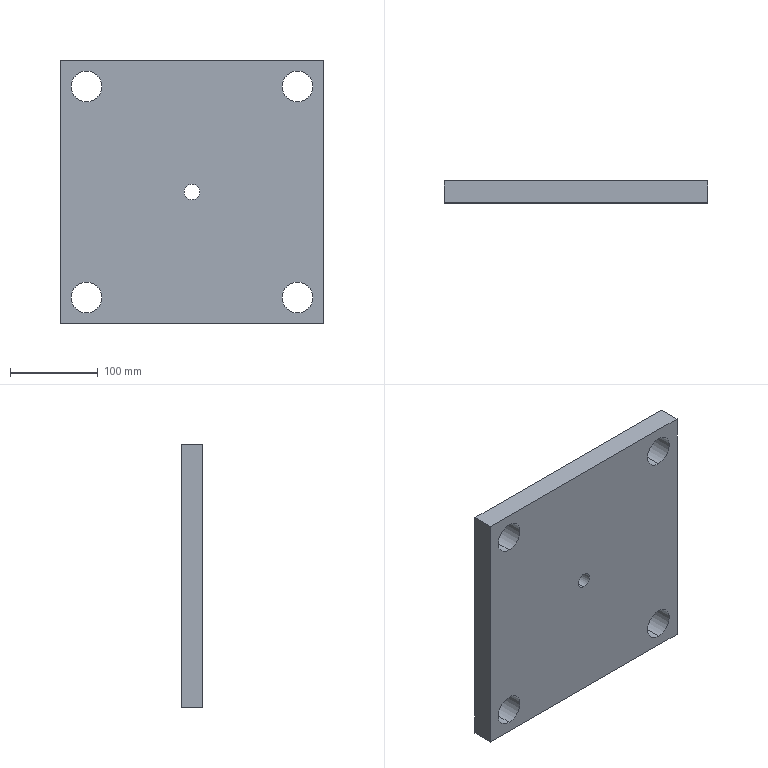Part | SolidWorks | features FlatPattern 1, SMBaseFlange 1, SheetMetal 1 | 1 solid | 16 faces | box 300 x 25 x 300 mm | volume 2147427 mm3 | cylinder 10 | plane 6 | commonest cylinder face diameters 35 x8 18 x2
STEP:
#1=CARTESIAN_POINT('',(-120.,-25.,-137.5));
#2=VERTEX_POINT('',#1);
#3=CARTESIAN_POINT('',(-120.,-25.,-102.5));
#4=VERTEX_POINT('',#3);
#5=CARTESIAN_POINT('',(-120.,-25.,-120.));
#6=DIRECTION('',(0.,1.,0.));
#7=DIRECTION('',(0.,0.,-1.));
#8=AXIS2_PLACEMENT_3D('',#5,#6,#7);
#9=CIRCLE('',#8,17.5);
#10=EDGE_CURVE('',#2,#4,#9,.T.);
#11=ORIENTED_EDGE('',*,*,#10,.F.);
#12=CARTESIAN_POINT('',(-120.,0.,-137.5));
#13=VERTEX_POINT('',#12);
#14=CARTESIAN_POINT('',(-120.,-25.,-137.5));
#15=DIRECTION('',(0.,1.,0.));
#16=VECTOR('',#15,1000.);
#17=LINE('',#14,#16);
#18=EDGE_CURVE('',#2,#13,#17,.T.);
#19=ORIENTED_EDGE('',*,*,#18,.T.);
#20=CARTESIAN_POINT('',(-120.,0.,-102.5));
#21=VERTEX_POINT('',#20);
#22=CARTESIAN_POINT('',(-120.,0.,-120.));
#23=DIRECTION('',(0.,1.,0.));
#24=DIRECTION('',(0.,0.,-1.));
#25=AXIS2_PLACEMENT_3D('',#22,#23,#24);
#26=CIRCLE('',#25,17.5);
#27=EDGE_CURVE('',#13,#21,#26,.T.);
#28=ORIENTED_EDGE('',*,*,#27,.T.);
#29=CARTESIAN_POINT('',(-120.,-25.,-102.5));
#30=DIRECTION('',(0.,1.,0.));
#31=VECTOR('',#30,1000.);
#32=LINE('',#29,#31);
#33=EDGE_CURVE('',#4,#21,#32,.T.);
#34=ORIENTED_EDGE('',*,*,#33,.F.);
#35=EDGE_LOOP('',(#11,#19,#28,#34));
#36=FACE_OUTER_BOUND('',#35,.T.);
#37=CARTESIAN_POINT('',(-120.,-25.,-120.));
#38=DIRECTION('',(0.,1.,0.));
#39=DIRECTION('',(0.,0.,1.));
#40=AXIS2_PLACEMENT_3D('',#37,#38,#39);
#41=CYLINDRICAL_SURFACE('',#40,17.5);
#42=ADVANCED_FACE('',(#36),#41,.F.);
#43=CARTESIAN_POINT('',(120.,-25.,-137.5));
#44=VERTEX_POINT('',#43);
#45=CARTESIAN_POINT('',(120.,-25.,-102.5));
#46=VERTEX_POINT('',#45);
#47=CARTESIAN_POINT('',(120.,-25.,-120.));
#48=DIRECTION('',(0.,1.,0.));
#49=DIRECTION('',(0.,0.,1.));
#50=AXIS2_PLACEMENT_3D('',#47,#48,#49);
#51=CIRCLE('',#50,17.5);
#52=EDGE_CURVE('',#44,#46,#51,.T.);
#53=ORIENTED_EDGE('',*,*,#52,.F.);
#54=CARTESIAN_POINT('',(120.,0.,-137.5));
#55=VERTEX_POINT('',#54);
#56=CARTESIAN_POINT('',(120.,-25.,-137.5));
#57=DIRECTION('',(0.,1.,0.));
#58=VECTOR('',#57,1000.);
#59=LINE('',#56,#58);
#60=EDGE_CURVE('',#44,#55,#59,.T.);
#61=ORIENTED_EDGE('',*,*,#60,.T.);
#62=CARTESIAN_POINT('',(120.,0.,-102.5));
#63=VERTEX_POINT('',#62);
#64=CARTESIAN_POINT('',(120.,0.,-120.));
#65=DIRECTION('',(0.,1.,0.));
#66=DIRECTION('',(0.,0.,1.));
#67=AXIS2_PLACEMENT_3D('',#64,#65,#66);
#68=CIRCLE('',#67,17.5);
#69=EDGE_CURVE('',#55,#63,#68,.T.);
#70=ORIENTED_EDGE('',*,*,#69,.T.);
#71=CARTESIAN_POINT('',(120.,-25.,-102.5));
#72=DIRECTION('',(0.,1.,0.));
#73=VECTOR('',#72,1000.);
#74=LINE('',#71,#73);
#75=EDGE_CURVE('',#46,#63,#74,.T.);
#76=ORIENTED_EDGE('',*,*,#75,.F.);
#77=EDGE_LOOP('',(#53,#61,#70,#76));
#78=FACE_OUTER_BOUND('',#77,.T.);
#79=CARTESIAN_POINT('',(120.,-25.,-120.));
#80=DIRECTION('',(0.,1.,0.));
#81=DIRECTION('',(0.,0.,1.));
#82=AXIS2_PLACEMENT_3D('',#79,#80,#81);
#83=CYLINDRICAL_SURFACE('',#82,17.5);
#84=ADVANCED_FACE('',(#78),#83,.F.);
#85=CARTESIAN_POINT('',(0.,-25.,-9.));
#86=VERTEX_POINT('',#85);
#87=CARTESIAN_POINT('',(0.,-25.,9.));
#88=VERTEX_POINT('',#87);
#89=CARTESIAN_POINT('',(0.,-25.,0.));
#90=DIRECTION('',(0.,1.,0.));
#91=DIRECTION('',(0.,0.,1.));
#92=AXIS2_PLACEMENT_3D('',#89,#90,#91);
#93=CIRCLE('',#92,9.);
#94=EDGE_CURVE('',#86,#88,#93,.T.);
#95=ORIENTED_EDGE('',*,*,#94,.F.);
#96=CARTESIAN_POINT('',(0.,0.,-9.));
#97=VERTEX_POINT('',#96);
#98=CARTESIAN_POINT('',(0.,-25.,-9.));
#99=DIRECTION('',(0.,1.,0.));
#100=VECTOR('',#99,1000.);
#101=LINE('',#98,#100);
#102=EDGE_CURVE('',#86,#97,#101,.T.);
#103=ORIENTED_EDGE('',*,*,#102,.T.);
#104=CARTESIAN_POINT('',(0.,0.,9.));
#105=VERTEX_POINT('',#104);
#106=CARTESIAN_POINT('',(0.,0.,0.));
#107=DIRECTION('',(0.,1.,0.));
#108=DIRECTION('',(0.,0.,1.));
#109=AXIS2_PLACEMENT_3D('',#106,#107,#108);
#110=CIRCLE('',#109,9.);
#111=EDGE_CURVE('',#97,#105,#110,.T.);
#112=ORIENTED_EDGE('',*,*,#111,.T.);
#113=CARTESIAN_POINT('',(0.,-25.,9.));
#114=DIRECTION('',(0.,1.,0.));
#115=VECTOR('',#114,1000.);
#116=LINE('',#113,#115);
#117=EDGE_CURVE('',#88,#105,#116,.T.);
#118=ORIENTED_EDGE('',*,*,#117,.F.);
#119=EDGE_LOOP('',(#95,#103,#112,#118));
#120=FACE_OUTER_BOUND('',#119,.T.);
#121=CARTESIAN_POINT('',(0.,-25.,0.));
#122=DIRECTION('',(0.,1.,0.));
#123=DIRECTION('',(0.,0.,1.));
#124=AXIS2_PLACEMENT_3D('',#121,#122,#123);
#125=CYLINDRICAL_SURFACE('',#124,9.);
#126=ADVANCED_FACE('',(#120),#125,.F.);
#127=CARTESIAN_POINT('',(120.,-25.,102.5));
#128=VERTEX_POINT('',#127);
#129=CARTESIAN_POINT('',(120.,-25.,137.5));
#130=VERTEX_POINT('',#129);
#131=CARTESIAN_POINT('',(120.,-25.,120.));
#132=DIRECTION('',(0.,1.,0.));
#133=DIRECTION('',(0.,0.,-1.));
#134=AXIS2_PLACEMENT_3D('',#131,#132,#133);
#135=CIRCLE('',#134,17.5);
#136=EDGE_CURVE('',#128,#130,#135,.T.);
#137=ORIENTED_EDGE('',*,*,#136,.F.);
#138=CARTESIAN_POINT('',(120.,0.,102.5));
#139=VERTEX_POINT('',#138);
#140=CARTESIAN_POINT('',(120.,-25.,102.5));
#141=DIRECTION('',(0.,1.,0.));
#142=VECTOR('',#141,1000.);
#143=LINE('',#140,#142);
#144=EDGE_CURVE('',#128,#139,#143,.T.);
#145=ORIENTED_EDGE('',*,*,#144,.T.);
#146=CARTESIAN_POINT('',(120.,0.,137.5));
#147=VERTEX_POINT('',#146);
#148=CARTESIAN_POINT('',(120.,0.,120.));
#149=DIRECTION('',(0.,1.,0.));
#150=DIRECTION('',(0.,0.,-1.));
#151=AXIS2_PLACEMENT_3D('',#148,#149,#150);
#152=CIRCLE('',#151,17.5);
#153=EDGE_CURVE('',#139,#147,#152,.T.);
#154=ORIENTED_EDGE('',*,*,#153,.T.);
#155=CARTESIAN_POINT('',(120.,-25.,137.5));
#156=DIRECTION('',(0.,1.,0.));
#157=VECTOR('',#156,1000.);
#158=LINE('',#155,#157);
#159=EDGE_CURVE('',#130,#147,#158,.T.);
#160=ORIENTED_EDGE('',*,*,#159,.F.);
#161=EDGE_LOOP('',(#137,#145,#154,#160));
#162=FACE_OUTER_BOUND('',#161,.T.);
#163=CARTESIAN_POINT('',(120.,-25.,120.));
#164=DIRECTION('',(0.,1.,0.));
#165=DIRECTION('',(0.,0.,1.));
#166=AXIS2_PLACEMENT_3D('',#163,#164,#165);
#167=CYLINDRICAL_SURFACE('',#166,17.5);
#168=ADVANCED_FACE('',(#162),#167,.F.);
#169=CARTESIAN_POINT('',(-120.,-25.,102.5));
#170=VERTEX_POINT('',#169);
#171=CARTESIAN_POINT('',(-120.,-25.,137.5));
#172=VERTEX_POINT('',#171);
#173=CARTESIAN_POINT('',(-120.,-25.,120.));
#174=DIRECTION('',(0.,1.,0.));
#175=DIRECTION('',(0.,0.,1.));
#176=AXIS2_PLACEMENT_3D('',#173,#174,#175);
#177=CIRCLE('',#176,17.5);
#178=EDGE_CURVE('',#170,#172,#177,.T.);
#179=ORIENTED_EDGE('',*,*,#178,.F.);
#180=CARTESIAN_POINT('',(-120.,0.,102.5));
#181=VERTEX_POINT('',#180);
#182=CARTESIAN_POINT('',(-120.,-25.,102.5));
#183=DIRECTION('',(0.,1.,0.));
#184=VECTOR('',#183,1000.);
#185=LINE('',#182,#184);
#186=EDGE_CURVE('',#170,#181,#185,.T.);
#187=ORIENTED_EDGE('',*,*,#186,.T.);
#188=CARTESIAN_POINT('',(-120.,0.,137.5));
#189=VERTEX_POINT('',#188);
#190=CARTESIAN_POINT('',(-120.,0.,120.));
#191=DIRECTION('',(0.,1.,0.));
#192=DIRECTION('',(0.,0.,1.));
#193=AXIS2_PLACEMENT_3D('',#190,#191,#192);
#194=CIRCLE('',#193,17.5);
#195=EDGE_CURVE('',#181,#189,#194,.T.);
#196=ORIENTED_EDGE('',*,*,#195,.T.);
#197=CARTESIAN_POINT('',(-120.,-25.,137.5));
#198=DIRECTION('',(0.,1.,0.));
#199=VECTOR('',#198,1000.);
#200=LINE('',#197,#199);
#201=EDGE_CURVE('',#172,#189,#200,.T.);
#202=ORIENTED_EDGE('',*,*,#201,.F.);
#203=EDGE_LOOP('',(#179,#187,#196,#202));
#204=FACE_OUTER_BOUND('',#203,.T.);
#205=CARTESIAN_POINT('',(-120.,-25.,120.));
#206=DIRECTION('',(0.,1.,0.));
#207=DIRECTION('',(0.,0.,1.));
#208=AXIS2_PLACEMENT_3D('',#205,#206,#207);
#209=CYLINDRICAL_SURFACE('',#208,17.5);
#210=ADVANCED_FACE('',(#204),#209,.F.);
#211=CARTESIAN_POINT('',(150.,0.,150.));
#212=VERTEX_POINT('',#211);
#213=CARTESIAN_POINT('',(150.,0.,-150.));
#214=VERTEX_POINT('',#213);
#215=CARTESIAN_POINT('',(150.,0.,-150.));
#216=DIRECTION('',(0.,0.,-1.));
#217=VECTOR('',#216,1000.);
#218=LINE('',#215,#217);
#219=EDGE_CURVE('',#212,#214,#218,.T.);
#220=ORIENTED_EDGE('',*,*,#219,.F.);
#221=CARTESIAN_POINT('',(150.,-25.,150.));
#222=VERTEX_POINT('',#221);
#223=CARTESIAN_POINT('',(150.,-25.,150.));
#224=DIRECTION('',(0.,1.,0.));
#225=VECTOR('',#224,1000.);
#226=LINE('',#223,#225);
#227=EDGE_CURVE('',#222,#212,#226,.T.);
#228=ORIENTED_EDGE('',*,*,#227,.F.);
#229=CARTESIAN_POINT('',(150.,-25.,-150.));
#230=VERTEX_POINT('',#229);
#231=CARTESIAN_POINT('',(150.,-25.,-150.));
#232=DIRECTION('',(0.,0.,-1.));
#233=VECTOR('',#232,1000.);
#234=LINE('',#231,#233);
#235=EDGE_CURVE('',#222,#230,#234,.T.);
#236=ORIENTED_EDGE('',*,*,#235,.T.);
#237=CARTESIAN_POINT('',(150.,-25.,-150.));
#238=DIRECTION('',(0.,1.,0.));
#239=VECTOR('',#238,1000.);
#240=LINE('',#237,#239);
#241=EDGE_CURVE('',#230,#214,#240,.T.);
#242=ORIENTED_EDGE('',*,*,#241,.T.);
#243=EDGE_LOOP('',(#220,#228,#236,#242));
#244=FACE_OUTER_BOUND('',#243,.T.);
#245=CARTESIAN_POINT('',(150.,-25.,-150.));
#246=DIRECTION('',(1.,0.,0.));
#247=DIRECTION('',(0.,0.,-1.));
#248=AXIS2_PLACEMENT_3D('',#245,#246,#247);
#249=PLANE('',#248);
#250=ADVANCED_FACE('',(#244),#249,.T.);
#251=CARTESIAN_POINT('',(-150.,0.,150.));
#252=VERTEX_POINT('',#251);
#253=CARTESIAN_POINT('',(-150.,0.,150.));
#254=DIRECTION('',(1.,0.,0.));
#255=VECTOR('',#254,1000.);
#256=LINE('',#253,#255);
#257=EDGE_CURVE('',#252,#212,#256,.T.);
#258=ORIENTED_EDGE('',*,*,#257,.F.);
#259=CARTESIAN_POINT('',(-150.,-25.,150.));
#260=VERTEX_POINT('',#259);
#261=CARTESIAN_POINT('',(-150.,-25.,150.));
#262=DIRECTION('',(0.,1.,0.));
#263=VECTOR('',#262,1000.);
#264=LINE('',#261,#263);
#265=EDGE_CURVE('',#260,#252,#264,.T.);
#266=ORIENTED_EDGE('',*,*,#265,.F.);
#267=CARTESIAN_POINT('',(-150.,-25.,150.));
#268=DIRECTION('',(1.,0.,0.));
#269=VECTOR('',#268,1000.);
#270=LINE('',#267,#269);
#271=EDGE_CURVE('',#260,#222,#270,.T.);
#272=ORIENTED_EDGE('',*,*,#271,.T.);
#273=ORIENTED_EDGE('',*,*,#227,.T.);
#274=EDGE_LOOP('',(#258,#266,#272,#273));
#275=FACE_OUTER_BOUND('',#274,.T.);
#276=CARTESIAN_POINT('',(-150.,-25.,150.));
#277=DIRECTION('',(0.,0.,1.));
#278=DIRECTION('',(1.,0.,0.));
#279=AXIS2_PLACEMENT_3D('',#276,#277,#278);
#280=PLANE('',#279);
#281=ADVANCED_FACE('',(#275),#280,.T.);
#282=CARTESIAN_POINT('',(-150.,0.,-150.));
#283=VERTEX_POINT('',#282);
#284=CARTESIAN_POINT('',(-150.,0.,-150.));
#285=DIRECTION('',(0.,0.,1.));
#286=VECTOR('',#285,1000.);
#287=LINE('',#284,#286);
#288=EDGE_CURVE('',#283,#252,#287,.T.);
#289=ORIENTED_EDGE('',*,*,#288,.F.);
#290=CARTESIAN_POINT('',(-150.,-25.,-150.));
#291=VERTEX_POINT('',#290);
#292=CARTESIAN_POINT('',(-150.,-25.,-150.));
#293=DIRECTION('',(0.,1.,0.));
#294=VECTOR('',#293,1000.);
#295=LINE('',#292,#294);
#296=EDGE_CURVE('',#291,#283,#295,.T.);
#297=ORIENTED_EDGE('',*,*,#296,.F.);
#298=CARTESIAN_POINT('',(-150.,-25.,-150.));
#299=DIRECTION('',(0.,0.,1.));
#300=VECTOR('',#299,1000.);
#301=LINE('',#298,#300);
#302=EDGE_CURVE('',#291,#260,#301,.T.);
#303=ORIENTED_EDGE('',*,*,#302,.T.);
#304=ORIENTED_EDGE('',*,*,#265,.T.);
#305=EDGE_LOOP('',(#289,#297,#303,#304));
#306=FACE_OUTER_BOUND('',#305,.T.);
#307=CARTESIAN_POINT('',(-150.,-25.,-150.));
#308=DIRECTION('',(-1.,0.,0.));
#309=DIRECTION('',(0.,0.,1.));
#310=AXIS2_PLACEMENT_3D('',#307,#308,#309);
#311=PLANE('',#310);
#312=ADVANCED_FACE('',(#306),#311,.T.);
#313=CARTESIAN_POINT('',(-150.,0.,-150.));
#314=DIRECTION('',(-1.,0.,0.));
#315=VECTOR('',#314,1000.);
#316=LINE('',#313,#315);
#317=EDGE_CURVE('',#214,#283,#316,.T.);
#318=ORIENTED_EDGE('',*,*,#317,.F.);
#319=ORIENTED_EDGE('',*,*,#241,.F.);
#320=CARTESIAN_POINT('',(-150.,-25.,-150.));
#321=DIRECTION('',(-1.,0.,0.));
#322=VECTOR('',#321,1000.);
#323=LINE('',#320,#322);
#324=EDGE_CURVE('',#230,#291,#323,.T.);
#325=ORIENTED_EDGE('',*,*,#324,.T.);
#326=ORIENTED_EDGE('',*,*,#296,.T.);
#327=EDGE_LOOP('',(#318,#319,#325,#326));
#328=FACE_OUTER_BOUND('',#327,.T.);
#329=CARTESIAN_POINT('',(-150.,-25.,-150.));
#330=DIRECTION('',(0.,0.,-1.));
#331=DIRECTION('',(-1.,0.,0.));
#332=AXIS2_PLACEMENT_3D('',#329,#330,#331);
#333=PLANE('',#332);
#334=ADVANCED_FACE('',(#328),#333,.T.);
#335=CARTESIAN_POINT('',(-120.,-25.,-120.));
#336=DIRECTION('',(0.,1.,0.));
#337=DIRECTION('',(0.,0.,-1.));
#338=AXIS2_PLACEMENT_3D('',#335,#336,#337);
#339=CIRCLE('',#338,17.5);
#340=EDGE_CURVE('',#4,#2,#339,.T.);
#341=ORIENTED_EDGE('',*,*,#340,.T.);
#342=ORIENTED_EDGE('',*,*,#10,.T.);
#343=EDGE_LOOP('',(#341,#342));
#344=FACE_BOUND('',#343,.T.);
#345=CARTESIAN_POINT('',(120.,-25.,-120.));
#346=DIRECTION('',(0.,1.,0.));
#347=DIRECTION('',(0.,0.,1.));
#348=AXIS2_PLACEMENT_3D('',#345,#346,#347);
#349=CIRCLE('',#348,17.5);
#350=EDGE_CURVE('',#46,#44,#349,.T.);
#351=ORIENTED_EDGE('',*,*,#350,.T.);
#352=ORIENTED_EDGE('',*,*,#52,.T.);
#353=EDGE_LOOP('',(#351,#352));
#354=FACE_BOUND('',#353,.T.);
#355=CARTESIAN_POINT('',(0.,-25.,0.));
#356=DIRECTION('',(0.,1.,0.));
#357=DIRECTION('',(0.,0.,1.));
#358=AXIS2_PLACEMENT_3D('',#355,#356,#357);
#359=CIRCLE('',#358,9.);
#360=EDGE_CURVE('',#88,#86,#359,.T.);
#361=ORIENTED_EDGE('',*,*,#360,.T.);
#362=ORIENTED_EDGE('',*,*,#94,.T.);
#363=EDGE_LOOP('',(#361,#362));
#364=FACE_BOUND('',#363,.T.);
#365=CARTESIAN_POINT('',(120.,-25.,120.));
#366=DIRECTION('',(0.,1.,0.));
#367=DIRECTION('',(0.,0.,-1.));
#368=AXIS2_PLACEMENT_3D('',#365,#366,#367);
#369=CIRCLE('',#368,17.5);
#370=EDGE_CURVE('',#130,#128,#369,.T.);
#371=ORIENTED_EDGE('',*,*,#370,.T.);
#372=ORIENTED_EDGE('',*,*,#136,.T.);
#373=EDGE_LOOP('',(#371,#372));
#374=FACE_BOUND('',#373,.T.);
#375=CARTESIAN_POINT('',(-120.,-25.,120.));
#376=DIRECTION('',(0.,1.,0.));
#377=DIRECTION('',(0.,0.,1.));
#378=AXIS2_PLACEMENT_3D('',#375,#376,#377);
#379=CIRCLE('',#378,17.5);
#380=EDGE_CURVE('',#172,#170,#379,.T.);
#381=ORIENTED_EDGE('',*,*,#380,.T.);
#382=ORIENTED_EDGE('',*,*,#178,.T.);
#383=EDGE_LOOP('',(#381,#382));
#384=FACE_BOUND('',#383,.T.);
#385=ORIENTED_EDGE('',*,*,#235,.F.);
#386=ORIENTED_EDGE('',*,*,#271,.F.);
#387=ORIENTED_EDGE('',*,*,#302,.F.);
#388=ORIENTED_EDGE('',*,*,#324,.F.);
#389=EDGE_LOOP('',(#385,#386,#387,#388));
#390=FACE_OUTER_BOUND('',#389,.T.);
#391=CARTESIAN_POINT('',(0.,-25.,0.));
#392=DIRECTION('',(0.,1.,0.));
#393=DIRECTION('',(0.,0.,1.));
#394=AXIS2_PLACEMENT_3D('',#391,#392,#393);
#395=PLANE('',#394);
#396=ADVANCED_FACE('',(#344,#354,#364,#374,#384,#390),#395,.F.);
#397=CARTESIAN_POINT('',(-120.,0.,-120.));
#398=DIRECTION('',(0.,1.,0.));
#399=DIRECTION('',(0.,0.,-1.));
#400=AXIS2_PLACEMENT_3D('',#397,#398,#399);
#401=CIRCLE('',#400,17.5);
#402=EDGE_CURVE('',#21,#13,#401,.T.);
#403=ORIENTED_EDGE('',*,*,#402,.F.);
#404=ORIENTED_EDGE('',*,*,#27,.F.);
#405=EDGE_LOOP('',(#403,#404));
#406=FACE_BOUND('',#405,.T.);
#407=CARTESIAN_POINT('',(120.,0.,-120.));
#408=DIRECTION('',(0.,1.,0.));
#409=DIRECTION('',(0.,0.,1.));
#410=AXIS2_PLACEMENT_3D('',#407,#408,#409);
#411=CIRCLE('',#410,17.5);
#412=EDGE_CURVE('',#63,#55,#411,.T.);
#413=ORIENTED_EDGE('',*,*,#412,.F.);
#414=ORIENTED_EDGE('',*,*,#69,.F.);
#415=EDGE_LOOP('',(#413,#414));
#416=FACE_BOUND('',#415,.T.);
#417=CARTESIAN_POINT('',(0.,0.,0.));
#418=DIRECTION('',(0.,1.,0.));
#419=DIRECTION('',(0.,0.,1.));
#420=AXIS2_PLACEMENT_3D('',#417,#418,#419);
#421=CIRCLE('',#420,9.);
#422=EDGE_CURVE('',#105,#97,#421,.T.);
#423=ORIENTED_EDGE('',*,*,#422,.F.);
#424=ORIENTED_EDGE('',*,*,#111,.F.);
#425=EDGE_LOOP('',(#423,#424));
#426=FACE_BOUND('',#425,.T.);
#427=CARTESIAN_POINT('',(120.,0.,120.));
#428=DIRECTION('',(0.,1.,0.));
#429=DIRECTION('',(0.,0.,-1.));
#430=AXIS2_PLACEMENT_3D('',#427,#428,#429);
#431=CIRCLE('',#430,17.5);
#432=EDGE_CURVE('',#147,#139,#431,.T.);
#433=ORIENTED_EDGE('',*,*,#432,.F.);
#434=ORIENTED_EDGE('',*,*,#153,.F.);
#435=EDGE_LOOP('',(#433,#434));
#436=FACE_BOUND('',#435,.T.);
#437=CARTESIAN_POINT('',(-120.,0.,120.));
#438=DIRECTION('',(0.,1.,0.));
#439=DIRECTION('',(0.,0.,1.));
#440=AXIS2_PLACEMENT_3D('',#437,#438,#439);
#441=CIRCLE('',#440,17.5);
#442=EDGE_CURVE('',#189,#181,#441,.T.);
#443=ORIENTED_EDGE('',*,*,#442,.F.);
#444=ORIENTED_EDGE('',*,*,#195,.F.);
#445=EDGE_LOOP('',(#443,#444));
#446=FACE_BOUND('',#445,.T.);
#447=ORIENTED_EDGE('',*,*,#219,.T.);
#448=ORIENTED_EDGE('',*,*,#317,.T.);
#449=ORIENTED_EDGE('',*,*,#288,.T.);
#450=ORIENTED_EDGE('',*,*,#257,.T.);
#451=EDGE_LOOP('',(#447,#448,#449,#450));
#452=FACE_OUTER_BOUND('',#451,.T.);
#453=CARTESIAN_POINT('',(0.,0.,0.));
#454=DIRECTION('',(0.,1.,0.));
#455=DIRECTION('',(0.,0.,1.));
#456=AXIS2_PLACEMENT_3D('',#453,#454,#455);
#457=PLANE('',#456);
#458=ADVANCED_FACE('',(#406,#416,#426,#436,#446,#452),#457,.T.);
#459=ORIENTED_EDGE('',*,*,#186,.F.);
#460=ORIENTED_EDGE('',*,*,#380,.F.);
#461=ORIENTED_EDGE('',*,*,#201,.T.);
#462=ORIENTED_EDGE('',*,*,#442,.T.);
#463=EDGE_LOOP('',(#459,#460,#461,#462));
#464=FACE_OUTER_BOUND('',#463,.T.);
#465=CARTESIAN_POINT('',(-120.,-25.,120.));
#466=DIRECTION('',(0.,1.,0.));
#467=DIRECTION('',(0.,0.,1.));
#468=AXIS2_PLACEMENT_3D('',#465,#466,#467);
#469=CYLINDRICAL_SURFACE('',#468,17.5);
#470=ADVANCED_FACE('',(#464),#469,.F.);
#471=ORIENTED_EDGE('',*,*,#144,.F.);
#472=ORIENTED_EDGE('',*,*,#370,.F.);
#473=ORIENTED_EDGE('',*,*,#159,.T.);
#474=ORIENTED_EDGE('',*,*,#432,.T.);
#475=EDGE_LOOP('',(#471,#472,#473,#474));
#476=FACE_OUTER_BOUND('',#475,.T.);
#477=CARTESIAN_POINT('',(120.,-25.,120.));
#478=DIRECTION('',(0.,1.,0.));
#479=DIRECTION('',(0.,0.,1.));
#480=AXIS2_PLACEMENT_3D('',#477,#478,#479);
#481=CYLINDRICAL_SURFACE('',#480,17.5);
#482=ADVANCED_FACE('',(#476),#481,.F.);
#483=ORIENTED_EDGE('',*,*,#102,.F.);
#484=ORIENTED_EDGE('',*,*,#360,.F.);
#485=ORIENTED_EDGE('',*,*,#117,.T.);
#486=ORIENTED_EDGE('',*,*,#422,.T.);
#487=EDGE_LOOP('',(#483,#484,#485,#486));
#488=FACE_OUTER_BOUND('',#487,.T.);
#489=CARTESIAN_POINT('',(0.,-25.,0.));
#490=DIRECTION('',(0.,1.,0.));
#491=DIRECTION('',(0.,0.,1.));
#492=AXIS2_PLACEMENT_3D('',#489,#490,#491);
#493=CYLINDRICAL_SURFACE('',#492,9.);
#494=ADVANCED_FACE('',(#488),#493,.F.);
#495=ORIENTED_EDGE('',*,*,#60,.F.);
#496=ORIENTED_EDGE('',*,*,#350,.F.);
#497=ORIENTED_EDGE('',*,*,#75,.T.);
#498=ORIENTED_EDGE('',*,*,#412,.T.);
#499=EDGE_LOOP('',(#495,#496,#497,#498));
#500=FACE_OUTER_BOUND('',#499,.T.);
#501=CARTESIAN_POINT('',(120.,-25.,-120.));
#502=DIRECTION('',(0.,1.,0.));
#503=DIRECTION('',(0.,0.,1.));
#504=AXIS2_PLACEMENT_3D('',#501,#502,#503);
#505=CYLINDRICAL_SURFACE('',#504,17.5);
#506=ADVANCED_FACE('',(#500),#505,.F.);
#507=ORIENTED_EDGE('',*,*,#18,.F.);
#508=ORIENTED_EDGE('',*,*,#340,.F.);
#509=ORIENTED_EDGE('',*,*,#33,.T.);
#510=ORIENTED_EDGE('',*,*,#402,.T.);
#511=EDGE_LOOP('',(#507,#508,#509,#510));
#512=FACE_OUTER_BOUND('',#511,.T.);
#513=CARTESIAN_POINT('',(-120.,-25.,-120.));
#514=DIRECTION('',(0.,1.,0.));
#515=DIRECTION('',(0.,0.,1.));
#516=AXIS2_PLACEMENT_3D('',#513,#514,#515);
#517=CYLINDRICAL_SURFACE('',#516,17.5);
#518=ADVANCED_FACE('',(#512),#517,.F.);
#519=CLOSED_SHELL('',(#42,#84,#126,#168,#210,#250,#281,#312,#334,#396,#458,#470,#482,#494,#506,#518));
#520=MANIFOLD_SOLID_BREP('',#519);
#521=CARTESIAN_POINT('',(0.,0.,0.));
#522=DIRECTION('',(0.,0.,1.));
#523=DIRECTION('',(1.,0.,0.));
#524=AXIS2_PLACEMENT_3D('',#521,#522,#523);
#525=(LENGTH_UNIT()NAMED_UNIT(*)SI_UNIT(.MILLI.,.METRE.));
#526=UNCERTAINTY_MEASURE_WITH_UNIT(LENGTH_MEASURE(0.00001),#525,'','');
#527=(NAMED_UNIT(*)PLANE_ANGLE_UNIT()SI_UNIT($,.RADIAN.));
#528=(NAMED_UNIT(*)SI_UNIT($,.STERADIAN.)SOLID_ANGLE_UNIT());
#529=(GEOMETRIC_REPRESENTATION_CONTEXT(3)GLOBAL_UNCERTAINTY_ASSIGNED_CONTEXT((#526))GLOBAL_UNIT_ASSIGNED_CONTEXT((#525,#527,#528))REPRESENTATION_CONTEXT('',''));
#530=ADVANCED_BREP_SHAPE_REPRESENTATION('',(#520,#524),#529);